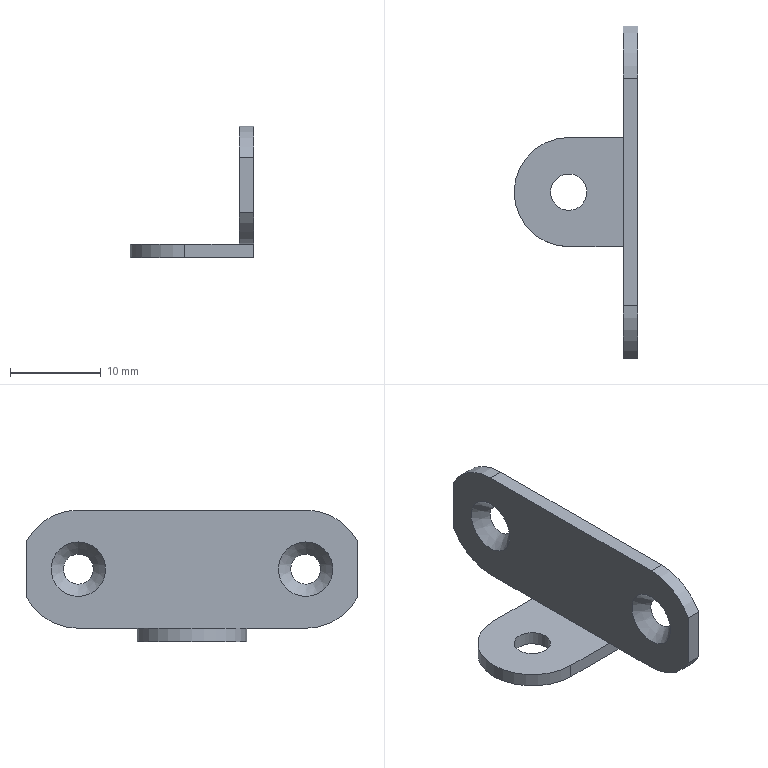Part | NX | 1 solid | 19 faces | box 13.6 x 36.5 x 14.5 mm | volume 869.458 mm3 | plane 11 | cylinder 6 | cone 2 | commonest cylinder face diameters 13 x4 4 x1 12 x1
STEP:
#1=CARTESIAN_POINT('',(7.6,12.5,9.65));
#2=VERTEX_POINT('',#1);
#3=CARTESIAN_POINT('',(7.6,12.5,8.));
#4=DIRECTION('',(-1.,0.,0.));
#5=DIRECTION('',(0.,0.,1.));
#6=AXIS2_PLACEMENT_3D('',#3,#4,#5);
#7=CIRCLE('',#6,1.65);
#8=EDGE_CURVE('',#2,#2,#7,.T.);
#9=ORIENTED_EDGE('',*,*,#8,.T.);
#10=EDGE_LOOP('',(#9));
#11=FACE_BOUND('',#10,.T.);
#12=CARTESIAN_POINT('',(7.6,18.25,11.031));
#13=VERTEX_POINT('',#12);
#14=CARTESIAN_POINT('',(7.6,18.25,4.969));
#15=VERTEX_POINT('',#14);
#16=CARTESIAN_POINT('',(7.6,18.25,14.5));
#17=DIRECTION('',(0.,0.,-1.));
#18=VECTOR('',#17,1000.);
#19=LINE('',#16,#18);
#20=EDGE_CURVE('',#13,#15,#19,.T.);
#21=ORIENTED_EDGE('',*,*,#20,.F.);
#22=CARTESIAN_POINT('',(7.6,12.5,14.5));
#23=VERTEX_POINT('',#22);
#24=CARTESIAN_POINT('',(7.6,12.5,8.));
#25=DIRECTION('',(-1.,0.,0.));
#26=DIRECTION('',(0.,0.,1.));
#27=AXIS2_PLACEMENT_3D('',#24,#25,#26);
#28=CIRCLE('',#27,6.5);
#29=EDGE_CURVE('',#13,#23,#28,.F.);
#30=ORIENTED_EDGE('',*,*,#29,.T.);
#31=CARTESIAN_POINT('',(7.6,-12.5,14.5));
#32=VERTEX_POINT('',#31);
#33=CARTESIAN_POINT('',(7.6,-18.25,14.5));
#34=DIRECTION('',(0.,1.,0.));
#35=VECTOR('',#34,1000.);
#36=LINE('',#33,#35);
#37=EDGE_CURVE('',#32,#23,#36,.T.);
#38=ORIENTED_EDGE('',*,*,#37,.F.);
#39=CARTESIAN_POINT('',(7.6,-18.25,11.031));
#40=VERTEX_POINT('',#39);
#41=CARTESIAN_POINT('',(7.6,-12.5,8.));
#42=DIRECTION('',(-1.,0.,0.));
#43=DIRECTION('',(0.,0.,1.));
#44=AXIS2_PLACEMENT_3D('',#41,#42,#43);
#45=CIRCLE('',#44,6.5);
#46=EDGE_CURVE('',#32,#40,#45,.F.);
#47=ORIENTED_EDGE('',*,*,#46,.T.);
#48=CARTESIAN_POINT('',(7.6,-18.25,4.969));
#49=VERTEX_POINT('',#48);
#50=CARTESIAN_POINT('',(7.6,-18.25,14.5));
#51=DIRECTION('',(0.,0.,-1.));
#52=VECTOR('',#51,1000.);
#53=LINE('',#50,#52);
#54=EDGE_CURVE('',#40,#49,#53,.T.);
#55=ORIENTED_EDGE('',*,*,#54,.T.);
#56=CARTESIAN_POINT('',(7.6,-12.5,1.5));
#57=VERTEX_POINT('',#56);
#58=CARTESIAN_POINT('',(7.6,-12.5,8.));
#59=DIRECTION('',(-1.,0.,0.));
#60=DIRECTION('',(0.,0.,1.));
#61=AXIS2_PLACEMENT_3D('',#58,#59,#60);
#62=CIRCLE('',#61,6.5);
#63=EDGE_CURVE('',#49,#57,#62,.F.);
#64=ORIENTED_EDGE('',*,*,#63,.T.);
#65=CARTESIAN_POINT('',(7.6,-6.,1.5));
#66=VERTEX_POINT('',#65);
#67=CARTESIAN_POINT('',(7.6,-18.25,1.5));
#68=DIRECTION('',(0.,1.,0.));
#69=VECTOR('',#68,1000.);
#70=LINE('',#67,#69);
#71=EDGE_CURVE('',#57,#66,#70,.T.);
#72=ORIENTED_EDGE('',*,*,#71,.T.);
#73=CARTESIAN_POINT('',(7.6,-6.,0.));
#74=VERTEX_POINT('',#73);
#75=CARTESIAN_POINT('',(7.6,-6.,14.5));
#76=DIRECTION('',(0.,0.,-1.));
#77=VECTOR('',#76,1000.);
#78=LINE('',#75,#77);
#79=EDGE_CURVE('',#66,#74,#78,.T.);
#80=ORIENTED_EDGE('',*,*,#79,.T.);
#81=CARTESIAN_POINT('',(7.6,6.,0.));
#82=VERTEX_POINT('',#81);
#83=CARTESIAN_POINT('',(7.6,-18.25,0.));
#84=DIRECTION('',(0.,1.,0.));
#85=VECTOR('',#84,1000.);
#86=LINE('',#83,#85);
#87=EDGE_CURVE('',#74,#82,#86,.T.);
#88=ORIENTED_EDGE('',*,*,#87,.T.);
#89=CARTESIAN_POINT('',(7.6,6.,1.5));
#90=VERTEX_POINT('',#89);
#91=CARTESIAN_POINT('',(7.6,6.,14.5));
#92=DIRECTION('',(0.,0.,1.));
#93=VECTOR('',#92,1000.);
#94=LINE('',#91,#93);
#95=EDGE_CURVE('',#82,#90,#94,.T.);
#96=ORIENTED_EDGE('',*,*,#95,.T.);
#97=CARTESIAN_POINT('',(7.6,12.5,1.5));
#98=VERTEX_POINT('',#97);
#99=CARTESIAN_POINT('',(7.6,-18.25,1.5));
#100=DIRECTION('',(0.,1.,0.));
#101=VECTOR('',#100,1000.);
#102=LINE('',#99,#101);
#103=EDGE_CURVE('',#90,#98,#102,.T.);
#104=ORIENTED_EDGE('',*,*,#103,.T.);
#105=CARTESIAN_POINT('',(7.6,12.5,8.));
#106=DIRECTION('',(-1.,0.,0.));
#107=DIRECTION('',(0.,0.,1.));
#108=AXIS2_PLACEMENT_3D('',#105,#106,#107);
#109=CIRCLE('',#108,6.5);
#110=EDGE_CURVE('',#98,#15,#109,.F.);
#111=ORIENTED_EDGE('',*,*,#110,.T.);
#112=EDGE_LOOP('',(#21,#30,#38,#47,#55,#64,#72,#80,#88,#96,#104,#111));
#113=FACE_BOUND('',#112,.T.);
#114=CARTESIAN_POINT('',(7.6,-12.5,9.65));
#115=VERTEX_POINT('',#114);
#116=CARTESIAN_POINT('',(7.6,-12.5,8.));
#117=DIRECTION('',(-1.,0.,0.));
#118=DIRECTION('',(0.,0.,1.));
#119=AXIS2_PLACEMENT_3D('',#116,#117,#118);
#120=CIRCLE('',#119,1.65);
#121=EDGE_CURVE('',#115,#115,#120,.T.);
#122=ORIENTED_EDGE('',*,*,#121,.T.);
#123=EDGE_LOOP('',(#122));
#124=FACE_BOUND('',#123,.T.);
#125=CARTESIAN_POINT('',(7.6,-18.25,14.5));
#126=DIRECTION('',(-1.,0.,0.));
#127=DIRECTION('',(0.,0.,1.));
#128=AXIS2_PLACEMENT_3D('',#125,#126,#127);
#129=PLANE('',#128);
#130=ADVANCED_FACE('',(#11,#113,#124),#129,.F.);
#131=CARTESIAN_POINT('',(6.,12.5,11.));
#132=VERTEX_POINT('',#131);
#133=CARTESIAN_POINT('',(6.,12.5,8.));
#134=DIRECTION('',(-1.,0.,0.));
#135=DIRECTION('',(0.,0.,1.));
#136=AXIS2_PLACEMENT_3D('',#133,#134,#135);
#137=CIRCLE('',#136,3.);
#138=EDGE_CURVE('',#132,#132,#137,.T.);
#139=ORIENTED_EDGE('',*,*,#138,.F.);
#140=EDGE_LOOP('',(#139));
#141=FACE_BOUND('',#140,.T.);
#142=CARTESIAN_POINT('',(6.,12.5,14.5));
#143=VERTEX_POINT('',#142);
#144=CARTESIAN_POINT('',(6.,-12.5,14.5));
#145=VERTEX_POINT('',#144);
#146=CARTESIAN_POINT('',(6.,-6.,14.5));
#147=DIRECTION('',(0.,-1.,0.));
#148=VECTOR('',#147,1000.);
#149=LINE('',#146,#148);
#150=EDGE_CURVE('',#143,#145,#149,.T.);
#151=ORIENTED_EDGE('',*,*,#150,.F.);
#152=CARTESIAN_POINT('',(6.,18.25,11.031));
#153=VERTEX_POINT('',#152);
#154=CARTESIAN_POINT('',(6.,12.5,8.));
#155=DIRECTION('',(1.,0.,0.));
#156=DIRECTION('',(0.,0.,-1.));
#157=AXIS2_PLACEMENT_3D('',#154,#155,#156);
#158=CIRCLE('',#157,6.5);
#159=EDGE_CURVE('',#143,#153,#158,.F.);
#160=ORIENTED_EDGE('',*,*,#159,.T.);
#161=CARTESIAN_POINT('',(6.,18.25,4.969));
#162=VERTEX_POINT('',#161);
#163=CARTESIAN_POINT('',(6.,18.25,14.5));
#164=DIRECTION('',(0.,0.,-1.));
#165=VECTOR('',#164,1000.);
#166=LINE('',#163,#165);
#167=EDGE_CURVE('',#153,#162,#166,.T.);
#168=ORIENTED_EDGE('',*,*,#167,.T.);
#169=CARTESIAN_POINT('',(6.,12.5,1.5));
#170=VERTEX_POINT('',#169);
#171=CARTESIAN_POINT('',(6.,12.5,8.));
#172=DIRECTION('',(1.,0.,0.));
#173=DIRECTION('',(0.,0.,-1.));
#174=AXIS2_PLACEMENT_3D('',#171,#172,#173);
#175=CIRCLE('',#174,6.5);
#176=EDGE_CURVE('',#162,#170,#175,.F.);
#177=ORIENTED_EDGE('',*,*,#176,.T.);
#178=CARTESIAN_POINT('',(6.,6.,1.5));
#179=VERTEX_POINT('',#178);
#180=CARTESIAN_POINT('',(6.,18.25,1.5));
#181=DIRECTION('',(0.,-1.,0.));
#182=VECTOR('',#181,1000.);
#183=LINE('',#180,#182);
#184=EDGE_CURVE('',#170,#179,#183,.T.);
#185=ORIENTED_EDGE('',*,*,#184,.T.);
#186=CARTESIAN_POINT('',(6.,-6.,1.5));
#187=VERTEX_POINT('',#186);
#188=CARTESIAN_POINT('',(6.,-14.5,1.5));
#189=DIRECTION('',(0.,1.,0.));
#190=VECTOR('',#189,1000.);
#191=LINE('',#188,#190);
#192=EDGE_CURVE('',#187,#179,#191,.T.);
#193=ORIENTED_EDGE('',*,*,#192,.F.);
#194=CARTESIAN_POINT('',(6.,-12.5,1.5));
#195=VERTEX_POINT('',#194);
#196=CARTESIAN_POINT('',(6.,18.25,1.5));
#197=DIRECTION('',(0.,-1.,0.));
#198=VECTOR('',#197,1000.);
#199=LINE('',#196,#198);
#200=EDGE_CURVE('',#187,#195,#199,.T.);
#201=ORIENTED_EDGE('',*,*,#200,.T.);
#202=CARTESIAN_POINT('',(6.,-18.25,4.969));
#203=VERTEX_POINT('',#202);
#204=CARTESIAN_POINT('',(6.,-12.5,8.));
#205=DIRECTION('',(1.,0.,0.));
#206=DIRECTION('',(0.,0.,-1.));
#207=AXIS2_PLACEMENT_3D('',#204,#205,#206);
#208=CIRCLE('',#207,6.5);
#209=EDGE_CURVE('',#195,#203,#208,.F.);
#210=ORIENTED_EDGE('',*,*,#209,.T.);
#211=CARTESIAN_POINT('',(6.,-18.25,11.031));
#212=VERTEX_POINT('',#211);
#213=CARTESIAN_POINT('',(6.,-18.25,14.5));
#214=DIRECTION('',(0.,0.,-1.));
#215=VECTOR('',#214,1000.);
#216=LINE('',#213,#215);
#217=EDGE_CURVE('',#212,#203,#216,.T.);
#218=ORIENTED_EDGE('',*,*,#217,.F.);
#219=CARTESIAN_POINT('',(6.,-12.5,8.));
#220=DIRECTION('',(1.,0.,0.));
#221=DIRECTION('',(0.,0.,-1.));
#222=AXIS2_PLACEMENT_3D('',#219,#220,#221);
#223=CIRCLE('',#222,6.5);
#224=EDGE_CURVE('',#212,#145,#223,.F.);
#225=ORIENTED_EDGE('',*,*,#224,.T.);
#226=EDGE_LOOP('',(#151,#160,#168,#177,#185,#193,#201,#210,#218,#225));
#227=FACE_BOUND('',#226,.T.);
#228=CARTESIAN_POINT('',(6.,-12.5,11.));
#229=VERTEX_POINT('',#228);
#230=CARTESIAN_POINT('',(6.,-12.5,8.));
#231=DIRECTION('',(-1.,0.,0.));
#232=DIRECTION('',(0.,0.,1.));
#233=AXIS2_PLACEMENT_3D('',#230,#231,#232);
#234=CIRCLE('',#233,3.);
#235=EDGE_CURVE('',#229,#229,#234,.T.);
#236=ORIENTED_EDGE('',*,*,#235,.F.);
#237=EDGE_LOOP('',(#236));
#238=FACE_BOUND('',#237,.T.);
#239=CARTESIAN_POINT('',(6.,18.25,14.5));
#240=DIRECTION('',(1.,0.,0.));
#241=DIRECTION('',(0.,0.,-1.));
#242=AXIS2_PLACEMENT_3D('',#239,#240,#241);
#243=PLANE('',#242);
#244=ADVANCED_FACE('',(#141,#227,#238),#243,.F.);
#245=CARTESIAN_POINT('',(14.5,12.5,14.5));
#246=DIRECTION('',(-1.,0.,0.));
#247=VECTOR('',#246,1000.);
#248=LINE('',#245,#247);
#249=EDGE_CURVE('',#23,#143,#248,.T.);
#250=ORIENTED_EDGE('',*,*,#249,.T.);
#251=ORIENTED_EDGE('',*,*,#150,.T.);
#252=CARTESIAN_POINT('',(14.5,-12.5,14.5));
#253=DIRECTION('',(-1.,0.,0.));
#254=VECTOR('',#253,1000.);
#255=LINE('',#252,#254);
#256=EDGE_CURVE('',#32,#145,#255,.T.);
#257=ORIENTED_EDGE('',*,*,#256,.F.);
#258=ORIENTED_EDGE('',*,*,#37,.T.);
#259=EDGE_LOOP('',(#250,#251,#257,#258));
#260=FACE_BOUND('',#259,.T.);
#261=CARTESIAN_POINT('',(0.,0.,14.5));
#262=DIRECTION('',(0.,0.,1.));
#263=DIRECTION('',(1.,0.,0.));
#264=AXIS2_PLACEMENT_3D('',#261,#262,#263);
#265=PLANE('',#264);
#266=ADVANCED_FACE('',(#260),#265,.T.);
#267=CARTESIAN_POINT('',(2.,0.,0.));
#268=VERTEX_POINT('',#267);
#269=CARTESIAN_POINT('',(0.,0.,0.));
#270=DIRECTION('',(0.,0.,1.));
#271=DIRECTION('',(1.,0.,0.));
#272=AXIS2_PLACEMENT_3D('',#269,#270,#271);
#273=CIRCLE('',#272,2.);
#274=EDGE_CURVE('',#268,#268,#273,.T.);
#275=ORIENTED_EDGE('',*,*,#274,.T.);
#276=EDGE_LOOP('',(#275));
#277=FACE_BOUND('',#276,.T.);
#278=CARTESIAN_POINT('',(0.,-6.,0.));
#279=VERTEX_POINT('',#278);
#280=CARTESIAN_POINT('',(0.,-6.,0.));
#281=DIRECTION('',(1.,0.,0.));
#282=VECTOR('',#281,1000.);
#283=LINE('',#280,#282);
#284=EDGE_CURVE('',#279,#74,#283,.T.);
#285=ORIENTED_EDGE('',*,*,#284,.F.);
#286=CARTESIAN_POINT('',(0.,6.,0.));
#287=VERTEX_POINT('',#286);
#288=CARTESIAN_POINT('',(0.,0.,0.));
#289=DIRECTION('',(0.,0.,1.));
#290=DIRECTION('',(1.,0.,0.));
#291=AXIS2_PLACEMENT_3D('',#288,#289,#290);
#292=CIRCLE('',#291,6.);
#293=EDGE_CURVE('',#287,#279,#292,.T.);
#294=ORIENTED_EDGE('',*,*,#293,.F.);
#295=CARTESIAN_POINT('',(6.,6.,0.));
#296=DIRECTION('',(-1.,0.,0.));
#297=VECTOR('',#296,1000.);
#298=LINE('',#295,#297);
#299=EDGE_CURVE('',#82,#287,#298,.T.);
#300=ORIENTED_EDGE('',*,*,#299,.F.);
#301=ORIENTED_EDGE('',*,*,#87,.F.);
#302=EDGE_LOOP('',(#285,#294,#300,#301));
#303=FACE_BOUND('',#302,.T.);
#304=CARTESIAN_POINT('',(0.,0.,0.));
#305=DIRECTION('',(0.,0.,1.));
#306=DIRECTION('',(1.,0.,0.));
#307=AXIS2_PLACEMENT_3D('',#304,#305,#306);
#308=PLANE('',#307);
#309=ADVANCED_FACE('',(#277,#303),#308,.F.);
#310=CARTESIAN_POINT('',(0.,-6.,1.5));
#311=VERTEX_POINT('',#310);
#312=CARTESIAN_POINT('',(0.,6.,1.5));
#313=VERTEX_POINT('',#312);
#314=CARTESIAN_POINT('',(0.,0.,1.5));
#315=DIRECTION('',(0.,0.,-1.));
#316=DIRECTION('',(-1.,0.,0.));
#317=AXIS2_PLACEMENT_3D('',#314,#315,#316);
#318=CIRCLE('',#317,6.);
#319=EDGE_CURVE('',#311,#313,#318,.T.);
#320=ORIENTED_EDGE('',*,*,#319,.T.);
#321=CARTESIAN_POINT('',(0.,6.,14.5));
#322=DIRECTION('',(0.,0.,-1.));
#323=VECTOR('',#322,1000.);
#324=LINE('',#321,#323);
#325=EDGE_CURVE('',#313,#287,#324,.T.);
#326=ORIENTED_EDGE('',*,*,#325,.T.);
#327=ORIENTED_EDGE('',*,*,#293,.T.);
#328=CARTESIAN_POINT('',(0.,-6.,14.5));
#329=DIRECTION('',(0.,0.,-1.));
#330=VECTOR('',#329,1000.);
#331=LINE('',#328,#330);
#332=EDGE_CURVE('',#311,#279,#331,.T.);
#333=ORIENTED_EDGE('',*,*,#332,.F.);
#334=EDGE_LOOP('',(#320,#326,#327,#333));
#335=FACE_BOUND('',#334,.T.);
#336=CARTESIAN_POINT('',(0.,0.,14.5));
#337=DIRECTION('',(0.,0.,-1.));
#338=DIRECTION('',(-1.,0.,0.));
#339=AXIS2_PLACEMENT_3D('',#336,#337,#338);
#340=CYLINDRICAL_SURFACE('',#339,6.);
#341=ADVANCED_FACE('',(#335),#340,.T.);
#342=ORIENTED_EDGE('',*,*,#284,.T.);
#343=ORIENTED_EDGE('',*,*,#79,.F.);
#344=CARTESIAN_POINT('',(14.5,-6.,1.5));
#345=DIRECTION('',(-1.,0.,0.));
#346=VECTOR('',#345,1000.);
#347=LINE('',#344,#346);
#348=EDGE_CURVE('',#66,#187,#347,.T.);
#349=ORIENTED_EDGE('',*,*,#348,.T.);
#350=CARTESIAN_POINT('',(0.,-6.,1.5));
#351=DIRECTION('',(-1.,0.,0.));
#352=VECTOR('',#351,1000.);
#353=LINE('',#350,#352);
#354=EDGE_CURVE('',#187,#311,#353,.T.);
#355=ORIENTED_EDGE('',*,*,#354,.T.);
#356=ORIENTED_EDGE('',*,*,#332,.T.);
#357=EDGE_LOOP('',(#342,#343,#349,#355,#356));
#358=FACE_BOUND('',#357,.T.);
#359=CARTESIAN_POINT('',(0.,-6.,14.5));
#360=DIRECTION('',(0.,1.,0.));
#361=DIRECTION('',(0.,0.,1.));
#362=AXIS2_PLACEMENT_3D('',#359,#360,#361);
#363=PLANE('',#362);
#364=ADVANCED_FACE('',(#358),#363,.F.);
#365=ORIENTED_EDGE('',*,*,#217,.T.);
#366=CARTESIAN_POINT('',(14.5,-18.25,4.969));
#367=DIRECTION('',(-1.,0.,0.));
#368=VECTOR('',#367,1000.);
#369=LINE('',#366,#368);
#370=EDGE_CURVE('',#203,#49,#369,.F.);
#371=ORIENTED_EDGE('',*,*,#370,.T.);
#372=ORIENTED_EDGE('',*,*,#54,.F.);
#373=CARTESIAN_POINT('',(14.5,-18.25,11.031));
#374=DIRECTION('',(-1.,0.,0.));
#375=VECTOR('',#374,1000.);
#376=LINE('',#373,#375);
#377=EDGE_CURVE('',#40,#212,#376,.T.);
#378=ORIENTED_EDGE('',*,*,#377,.T.);
#379=EDGE_LOOP('',(#365,#371,#372,#378));
#380=FACE_BOUND('',#379,.T.);
#381=CARTESIAN_POINT('',(6.,-18.25,14.5));
#382=DIRECTION('',(0.,1.,0.));
#383=DIRECTION('',(0.,0.,1.));
#384=AXIS2_PLACEMENT_3D('',#381,#382,#383);
#385=PLANE('',#384);
#386=ADVANCED_FACE('',(#380),#385,.F.);
#387=ORIENTED_EDGE('',*,*,#167,.F.);
#388=CARTESIAN_POINT('',(14.5,18.25,11.031));
#389=DIRECTION('',(-1.,0.,0.));
#390=VECTOR('',#389,1000.);
#391=LINE('',#388,#390);
#392=EDGE_CURVE('',#153,#13,#391,.F.);
#393=ORIENTED_EDGE('',*,*,#392,.T.);
#394=ORIENTED_EDGE('',*,*,#20,.T.);
#395=CARTESIAN_POINT('',(14.5,18.25,4.969));
#396=DIRECTION('',(-1.,0.,0.));
#397=VECTOR('',#396,1000.);
#398=LINE('',#395,#397);
#399=EDGE_CURVE('',#15,#162,#398,.T.);
#400=ORIENTED_EDGE('',*,*,#399,.T.);
#401=EDGE_LOOP('',(#387,#393,#394,#400));
#402=FACE_BOUND('',#401,.T.);
#403=CARTESIAN_POINT('',(7.6,18.25,14.5));
#404=DIRECTION('',(0.,-1.,0.));
#405=DIRECTION('',(0.,0.,-1.));
#406=AXIS2_PLACEMENT_3D('',#403,#404,#405);
#407=PLANE('',#406);
#408=ADVANCED_FACE('',(#402),#407,.F.);
#409=ORIENTED_EDGE('',*,*,#325,.F.);
#410=CARTESIAN_POINT('',(6.,6.,1.5));
#411=DIRECTION('',(1.,0.,0.));
#412=VECTOR('',#411,1000.);
#413=LINE('',#410,#412);
#414=EDGE_CURVE('',#313,#179,#413,.T.);
#415=ORIENTED_EDGE('',*,*,#414,.T.);
#416=CARTESIAN_POINT('',(14.5,6.,1.5));
#417=DIRECTION('',(-1.,0.,0.));
#418=VECTOR('',#417,1000.);
#419=LINE('',#416,#418);
#420=EDGE_CURVE('',#90,#179,#419,.T.);
#421=ORIENTED_EDGE('',*,*,#420,.F.);
#422=ORIENTED_EDGE('',*,*,#95,.F.);
#423=ORIENTED_EDGE('',*,*,#299,.T.);
#424=EDGE_LOOP('',(#409,#415,#421,#422,#423));
#425=FACE_BOUND('',#424,.T.);
#426=CARTESIAN_POINT('',(6.,6.,14.5));
#427=DIRECTION('',(0.,-1.,0.));
#428=DIRECTION('',(0.,0.,-1.));
#429=AXIS2_PLACEMENT_3D('',#426,#427,#428);
#430=PLANE('',#429);
#431=ADVANCED_FACE('',(#425),#430,.F.);
#432=CARTESIAN_POINT('',(-2.,0.,1.5));
#433=VERTEX_POINT('',#432);
#434=CARTESIAN_POINT('',(0.,0.,1.5));
#435=DIRECTION('',(0.,0.,-1.));
#436=DIRECTION('',(-1.,0.,0.));
#437=AXIS2_PLACEMENT_3D('',#434,#435,#436);
#438=CIRCLE('',#437,2.);
#439=EDGE_CURVE('',#433,#433,#438,.T.);
#440=ORIENTED_EDGE('',*,*,#439,.F.);
#441=EDGE_LOOP('',(#440));
#442=FACE_BOUND('',#441,.T.);
#443=ORIENTED_EDGE('',*,*,#274,.F.);
#444=EDGE_LOOP('',(#443));
#445=FACE_BOUND('',#444,.T.);
#446=CARTESIAN_POINT('',(0.,0.,14.5));
#447=DIRECTION('',(0.,0.,-1.));
#448=DIRECTION('',(-1.,0.,0.));
#449=AXIS2_PLACEMENT_3D('',#446,#447,#448);
#450=CYLINDRICAL_SURFACE('',#449,2.);
#451=ADVANCED_FACE('',(#442,#445),#450,.F.);
#452=ORIENTED_EDGE('',*,*,#439,.T.);
#453=EDGE_LOOP('',(#452));
#454=FACE_BOUND('',#453,.T.);
#455=ORIENTED_EDGE('',*,*,#192,.T.);
#456=ORIENTED_EDGE('',*,*,#414,.F.);
#457=ORIENTED_EDGE('',*,*,#319,.F.);
#458=ORIENTED_EDGE('',*,*,#354,.F.);
#459=EDGE_LOOP('',(#455,#456,#457,#458));
#460=FACE_BOUND('',#459,.T.);
#461=CARTESIAN_POINT('',(6.,-14.5,1.5));
#462=DIRECTION('',(0.,0.,-1.));
#463=DIRECTION('',(-1.,0.,0.));
#464=AXIS2_PLACEMENT_3D('',#461,#462,#463);
#465=PLANE('',#464);
#466=ADVANCED_FACE('',(#454,#460),#465,.F.);
#467=ORIENTED_EDGE('',*,*,#420,.T.);
#468=ORIENTED_EDGE('',*,*,#184,.F.);
#469=CARTESIAN_POINT('',(14.5,12.5,1.5));
#470=DIRECTION('',(-1.,0.,0.));
#471=VECTOR('',#470,1000.);
#472=LINE('',#469,#471);
#473=EDGE_CURVE('',#98,#170,#472,.T.);
#474=ORIENTED_EDGE('',*,*,#473,.F.);
#475=ORIENTED_EDGE('',*,*,#103,.F.);
#476=EDGE_LOOP('',(#467,#468,#474,#475));
#477=FACE_BOUND('',#476,.T.);
#478=CARTESIAN_POINT('',(14.5,6.,1.5));
#479=DIRECTION('',(0.,0.,1.));
#480=DIRECTION('',(1.,0.,0.));
#481=AXIS2_PLACEMENT_3D('',#478,#479,#480);
#482=PLANE('',#481);
#483=ADVANCED_FACE('',(#477),#482,.F.);
#484=ORIENTED_EDGE('',*,*,#473,.T.);
#485=ORIENTED_EDGE('',*,*,#176,.F.);
#486=ORIENTED_EDGE('',*,*,#399,.F.);
#487=ORIENTED_EDGE('',*,*,#110,.F.);
#488=EDGE_LOOP('',(#484,#485,#486,#487));
#489=FACE_BOUND('',#488,.T.);
#490=CARTESIAN_POINT('',(14.5,12.5,8.));
#491=DIRECTION('',(-1.,0.,0.));
#492=DIRECTION('',(0.,0.,1.));
#493=AXIS2_PLACEMENT_3D('',#490,#491,#492);
#494=CYLINDRICAL_SURFACE('',#493,6.5);
#495=ADVANCED_FACE('',(#489),#494,.T.);
#496=CARTESIAN_POINT('',(14.5,-12.5,1.5));
#497=DIRECTION('',(-1.,0.,0.));
#498=VECTOR('',#497,1000.);
#499=LINE('',#496,#498);
#500=EDGE_CURVE('',#57,#195,#499,.T.);
#501=ORIENTED_EDGE('',*,*,#500,.T.);
#502=ORIENTED_EDGE('',*,*,#200,.F.);
#503=ORIENTED_EDGE('',*,*,#348,.F.);
#504=ORIENTED_EDGE('',*,*,#71,.F.);
#505=EDGE_LOOP('',(#501,#502,#503,#504));
#506=FACE_BOUND('',#505,.T.);
#507=CARTESIAN_POINT('',(14.5,-12.5,1.5));
#508=DIRECTION('',(0.,0.,1.));
#509=DIRECTION('',(1.,0.,0.));
#510=AXIS2_PLACEMENT_3D('',#507,#508,#509);
#511=PLANE('',#510);
#512=ADVANCED_FACE('',(#506),#511,.F.);
#513=ORIENTED_EDGE('',*,*,#370,.F.);
#514=ORIENTED_EDGE('',*,*,#209,.F.);
#515=ORIENTED_EDGE('',*,*,#500,.F.);
#516=ORIENTED_EDGE('',*,*,#63,.F.);
#517=EDGE_LOOP('',(#513,#514,#515,#516));
#518=FACE_BOUND('',#517,.T.);
#519=CARTESIAN_POINT('',(14.5,-12.5,8.));
#520=DIRECTION('',(-1.,0.,0.));
#521=DIRECTION('',(0.,0.,1.));
#522=AXIS2_PLACEMENT_3D('',#519,#520,#521);
#523=CYLINDRICAL_SURFACE('',#522,6.5);
#524=ADVANCED_FACE('',(#518),#523,.T.);
#525=ORIENTED_EDGE('',*,*,#256,.T.);
#526=ORIENTED_EDGE('',*,*,#224,.F.);
#527=ORIENTED_EDGE('',*,*,#377,.F.);
#528=ORIENTED_EDGE('',*,*,#46,.F.);
#529=EDGE_LOOP('',(#525,#526,#527,#528));
#530=FACE_BOUND('',#529,.T.);
#531=CARTESIAN_POINT('',(14.5,-12.5,8.));
#532=DIRECTION('',(-1.,0.,0.));
#533=DIRECTION('',(0.,0.,1.));
#534=AXIS2_PLACEMENT_3D('',#531,#532,#533);
#535=CYLINDRICAL_SURFACE('',#534,6.5);
#536=ADVANCED_FACE('',(#530),#535,.T.);
#537=ORIENTED_EDGE('',*,*,#392,.F.);
#538=ORIENTED_EDGE('',*,*,#159,.F.);
#539=ORIENTED_EDGE('',*,*,#249,.F.);
#540=ORIENTED_EDGE('',*,*,#29,.F.);
#541=EDGE_LOOP('',(#537,#538,#539,#540));
#542=FACE_BOUND('',#541,.T.);
#543=CARTESIAN_POINT('',(14.5,12.5,8.));
#544=DIRECTION('',(-1.,0.,0.));
#545=DIRECTION('',(0.,0.,1.));
#546=AXIS2_PLACEMENT_3D('',#543,#544,#545);
#547=CYLINDRICAL_SURFACE('',#546,6.5);
#548=ADVANCED_FACE('',(#542),#547,.T.);
#549=ORIENTED_EDGE('',*,*,#138,.T.);
#550=EDGE_LOOP('',(#549));
#551=FACE_BOUND('',#550,.T.);
#552=ORIENTED_EDGE('',*,*,#8,.F.);
#553=EDGE_LOOP('',(#552));
#554=FACE_BOUND('',#553,.T.);
#555=CARTESIAN_POINT('',(7.6,12.5,8.));
#556=DIRECTION('',(-1.,0.,0.));
#557=DIRECTION('',(0.,0.,1.));
#558=AXIS2_PLACEMENT_3D('',#555,#556,#557);
#559=CONICAL_SURFACE('',#558,1.65,0.7009);
#560=ADVANCED_FACE('',(#551,#554),#559,.F.);
#561=ORIENTED_EDGE('',*,*,#235,.T.);
#562=EDGE_LOOP('',(#561));
#563=FACE_BOUND('',#562,.T.);
#564=ORIENTED_EDGE('',*,*,#121,.F.);
#565=EDGE_LOOP('',(#564));
#566=FACE_BOUND('',#565,.T.);
#567=CARTESIAN_POINT('',(7.6,-12.5,8.));
#568=DIRECTION('',(-1.,0.,0.));
#569=DIRECTION('',(0.,0.,1.));
#570=AXIS2_PLACEMENT_3D('',#567,#568,#569);
#571=CONICAL_SURFACE('',#570,1.65,0.7009);
#572=ADVANCED_FACE('',(#563,#566),#571,.F.);
#573=CLOSED_SHELL('',(#130,#244,#266,#309,#341,#364,#386,#408,#431,#451,#466,#483,#495,#512,#524,#536,#548,#560,#572));
#574=MANIFOLD_SOLID_BREP('',#573);
#575=(LENGTH_UNIT()NAMED_UNIT(*)SI_UNIT(.MILLI.,.METRE.));
#576=UNCERTAINTY_MEASURE_WITH_UNIT(LENGTH_MEASURE(0.00001),#575,'','');
#577=(NAMED_UNIT(*)PLANE_ANGLE_UNIT()SI_UNIT($,.RADIAN.));
#578=(NAMED_UNIT(*)SI_UNIT($,.STERADIAN.)SOLID_ANGLE_UNIT());
#579=(GEOMETRIC_REPRESENTATION_CONTEXT(3)GLOBAL_UNCERTAINTY_ASSIGNED_CONTEXT((#576))GLOBAL_UNIT_ASSIGNED_CONTEXT((#575,#577,#578))REPRESENTATION_CONTEXT('',''));
#580=ADVANCED_BREP_SHAPE_REPRESENTATION('',(#574),#579);